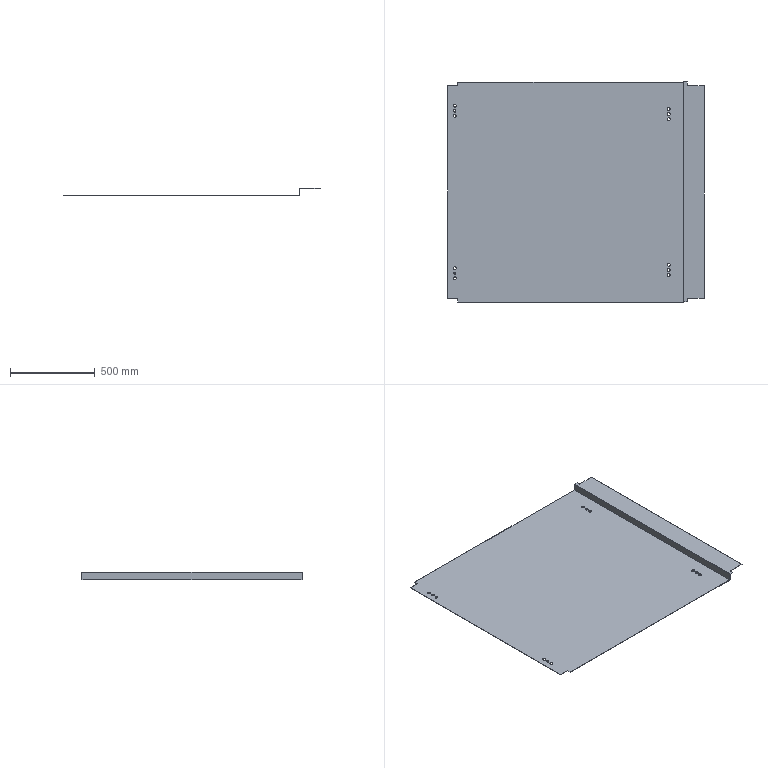Part | NX | features BREP 1 | 1 solid | 50 faces | box 1516 x 1300 x 44 mm | volume 4032528 mm3 | cylinder 26 | plane 24 | commonest cylinder face diameters 17 x20 12.5 x6